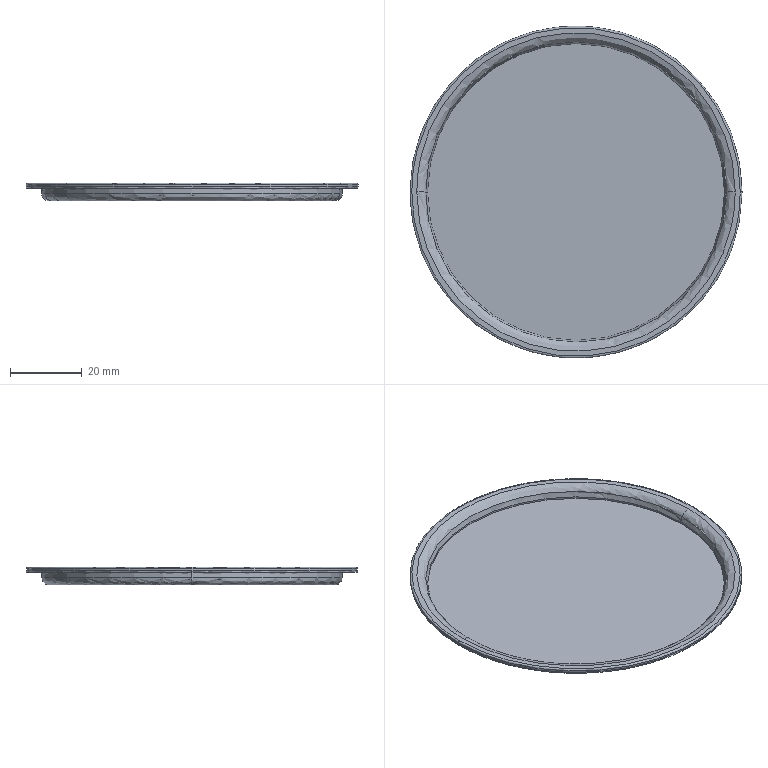Part | SolidWorks | features BaseBody 1 | 1 solid | 18 faces | box 92.8 x 92.8 x 5 mm | volume 9835 mm3 | spline 8 | cylinder 6 | plane 4 | commonest cylinder face diameters 83 x2 84 x2 92.8 x2
STEP:
#1=CARTESIAN_POINT('',(41.5,0.,2.));
#2=VERTEX_POINT('',#1);
#3=CARTESIAN_POINT('',(-41.5,0.,2.));
#4=VERTEX_POINT('',#3);
#5=CARTESIAN_POINT('',(0.,0.,2.));
#6=DIRECTION('',(0.,0.,-1.));
#7=DIRECTION('',(1.,0.,0.));
#8=AXIS2_PLACEMENT_3D('',#5,#6,#7);
#9=CIRCLE('',#8,41.5);
#10=EDGE_CURVE('',#2,#4,#9,.T.);
#11=ORIENTED_EDGE('',*,*,#10,.T.);
#12=CARTESIAN_POINT('',(-44.5,0.,5.));
#13=VERTEX_POINT('',#12);
#14=CARTESIAN_POINT('',(-44.5,0.,2.));
#15=DIRECTION('',(0.,-1.,0.));
#16=DIRECTION('',(-1.,0.,0.));
#17=AXIS2_PLACEMENT_3D('',#14,#15,#16);
#18=CIRCLE('',#17,3.);
#19=EDGE_CURVE('',#4,#13,#18,.T.);
#20=ORIENTED_EDGE('',*,*,#19,.T.);
#21=CARTESIAN_POINT('',(44.5,0.,5.));
#22=VERTEX_POINT('',#21);
#23=CARTESIAN_POINT('',(-44.5,0.,5.));
#24=CARTESIAN_POINT('',(-44.5,-89.,5.));
#25=CARTESIAN_POINT('',(44.5,-89.,5.));
#26=CARTESIAN_POINT('',(44.5,0.,5.));
#27=(BOUNDED_CURVE()B_SPLINE_CURVE(3,(#23,#24,#25,#26),.UNSPECIFIED.,.F.,.F.)B_SPLINE_CURVE_WITH_KNOTS((4,4),(0.,1.),.UNSPECIFIED.)CURVE()GEOMETRIC_REPRESENTATION_ITEM()RATIONAL_B_SPLINE_CURVE((1.,0.3333,0.3333,1.))REPRESENTATION_ITEM(''));
#28=EDGE_CURVE('',#13,#22,#27,.T.);
#29=ORIENTED_EDGE('',*,*,#28,.T.);
#30=CARTESIAN_POINT('',(44.5,0.,2.));
#31=DIRECTION('',(0.,1.,0.));
#32=DIRECTION('',(1.,0.,0.));
#33=AXIS2_PLACEMENT_3D('',#30,#31,#32);
#34=CIRCLE('',#33,3.);
#35=EDGE_CURVE('',#2,#22,#34,.T.);
#36=ORIENTED_EDGE('',*,*,#35,.F.);
#37=EDGE_LOOP('',(#11,#20,#29,#36));
#38=FACE_OUTER_BOUND('',#37,.T.);
#39=CARTESIAN_POINT('',(-41.5,0.,2.));
#40=CARTESIAN_POINT('',(-41.5,-83.,2.));
#41=CARTESIAN_POINT('',(41.5,-83.,2.));
#42=CARTESIAN_POINT('',(41.5,0.,2.));
#43=CARTESIAN_POINT('',(-41.5,0.,3.757));
#44=CARTESIAN_POINT('',(-41.5,-83.,3.757));
#45=CARTESIAN_POINT('',(41.5,-83.,3.757));
#46=CARTESIAN_POINT('',(41.5,0.,3.757));
#47=CARTESIAN_POINT('',(-42.743,0.,5.));
#48=CARTESIAN_POINT('',(-42.743,-85.485,5.));
#49=CARTESIAN_POINT('',(42.743,-85.485,5.));
#50=CARTESIAN_POINT('',(42.743,0.,5.));
#51=CARTESIAN_POINT('',(-44.5,0.,5.));
#52=CARTESIAN_POINT('',(-44.5,-89.,5.));
#53=CARTESIAN_POINT('',(44.5,-89.,5.));
#54=CARTESIAN_POINT('',(44.5,0.,5.));
#55=(BOUNDED_SURFACE()B_SPLINE_SURFACE(3,3,((#39,#40,#41,#42),(#43,#44,#45,#46),(#47,#48,#49,#50),(#51,#52,#53,#54)),.UNSPECIFIED.,.F.,.F.,.F.)B_SPLINE_SURFACE_WITH_KNOTS((4,4),(4,4),(0.,1.),(0.,1.),.UNSPECIFIED.)GEOMETRIC_REPRESENTATION_ITEM()RATIONAL_B_SPLINE_SURFACE(((1.,0.3333,0.3333,1.),(0.8047,0.2682,0.2682,0.8047),(0.8047,0.2682,0.2682,0.8047),(1.,0.3333,0.3333,1.)))REPRESENTATION_ITEM('')SURFACE());
#56=ADVANCED_FACE('',(#38),#55,.T.);
#57=CARTESIAN_POINT('',(-45.9,0.,5.));
#58=VERTEX_POINT('',#57);
#59=CARTESIAN_POINT('',(45.9,0.,5.));
#60=VERTEX_POINT('',#59);
#61=CARTESIAN_POINT('',(-45.9,0.,5.));
#62=CARTESIAN_POINT('',(-45.9,-1.404,5.));
#63=CARTESIAN_POINT('',(-45.804,-3.5,5.));
#64=CARTESIAN_POINT('',(-45.525,-5.931,5.));
#65=CARTESIAN_POINT('',(-45.343,-7.143,5.));
#66=CARTESIAN_POINT('',(-45.242,-7.748,5.));
#67=CARTESIAN_POINT('',(-45.189,-8.05,5.));
#68=CARTESIAN_POINT('',(-45.161,-8.201,5.));
#69=CARTESIAN_POINT('',(-45.15,-8.266,5.));
#70=CARTESIAN_POINT('',(-45.142,-8.309,5.));
#71=CARTESIAN_POINT('',(-45.138,-8.329,5.));
#72=CARTESIAN_POINT('',(-44.863,-9.816,5.));
#73=CARTESIAN_POINT('',(-44.353,-11.981,5.));
#74=CARTESIAN_POINT('',(-43.576,-14.456,5.));
#75=CARTESIAN_POINT('',(-43.142,-15.68,5.));
#76=CARTESIAN_POINT('',(-42.913,-16.289,5.));
#77=CARTESIAN_POINT('',(-42.796,-16.592,5.));
#78=CARTESIAN_POINT('',(-42.745,-16.722,5.));
#79=CARTESIAN_POINT('',(-42.711,-16.809,5.));
#80=CARTESIAN_POINT('',(-42.695,-16.85,5.));
#81=CARTESIAN_POINT('',(-42.106,-18.338,5.));
#82=CARTESIAN_POINT('',(-41.146,-20.447,5.));
#83=CARTESIAN_POINT('',(-39.843,-22.813,5.));
#84=CARTESIAN_POINT('',(-39.146,-23.973,5.));
#85=CARTESIAN_POINT('',(-38.786,-24.547,5.));
#86=CARTESIAN_POINT('',(-38.629,-24.792,5.));
#87=CARTESIAN_POINT('',(-38.524,-24.954,5.));
#88=CARTESIAN_POINT('',(-38.472,-25.034,5.));
#89=CARTESIAN_POINT('',(-36.684,-27.769,5.));
#90=CARTESIAN_POINT('',(-34.697,-30.216,5.));
#91=CARTESIAN_POINT('',(-31.336,-33.576,5.));
#92=CARTESIAN_POINT('',(-29.578,-35.162,5.));
#93=CARTESIAN_POINT('',(-27.393,-36.845,5.));
#94=CARTESIAN_POINT('',(-26.266,-37.646,5.));
#95=CARTESIAN_POINT('',(-25.694,-38.035,5.));
#96=CARTESIAN_POINT('',(-25.447,-38.2,5.));
#97=CARTESIAN_POINT('',(-25.283,-38.309,5.));
#98=CARTESIAN_POINT('',(-25.198,-38.365,5.));
#99=CARTESIAN_POINT('',(-23.819,-39.267,5.));
#100=CARTESIAN_POINT('',(-21.818,-40.436,5.));
#101=CARTESIAN_POINT('',(-19.388,-41.617,5.));
#102=CARTESIAN_POINT('',(-18.15,-42.162,5.));
#103=CARTESIAN_POINT('',(-17.525,-42.424,5.));
#104=CARTESIAN_POINT('',(-17.211,-42.551,5.));
#105=CARTESIAN_POINT('',(-17.076,-42.606,5.));
#106=CARTESIAN_POINT('',(-16.986,-42.642,5.));
#107=CARTESIAN_POINT('',(-16.939,-42.66,5.));
#108=CARTESIAN_POINT('',(-15.512,-43.225,5.));
#109=CARTESIAN_POINT('',(-13.406,-43.943,5.));
#110=CARTESIAN_POINT('',(-10.896,-44.599,5.));
#111=CARTESIAN_POINT('',(-9.629,-44.882,5.));
#112=CARTESIAN_POINT('',(-8.991,-45.011,5.));
#113=CARTESIAN_POINT('',(-8.672,-45.074,5.));
#114=CARTESIAN_POINT('',(-8.512,-45.104,5.));
#115=CARTESIAN_POINT('',(-8.444,-45.117,5.));
#116=CARTESIAN_POINT('',(-8.398,-45.125,5.));
#117=CARTESIAN_POINT('',(-8.374,-45.13,5.));
#118=CARTESIAN_POINT('',(-5.592,-45.645,5.));
#119=CARTESIAN_POINT('',(-2.807,-45.9,5.));
#120=CARTESIAN_POINT('',(1.404,-45.9,5.));
#121=CARTESIAN_POINT('',(3.5,-45.804,5.));
#122=CARTESIAN_POINT('',(5.931,-45.525,5.));
#123=CARTESIAN_POINT('',(7.143,-45.343,5.));
#124=CARTESIAN_POINT('',(7.748,-45.242,5.));
#125=CARTESIAN_POINT('',(8.05,-45.189,5.));
#126=CARTESIAN_POINT('',(8.201,-45.161,5.));
#127=CARTESIAN_POINT('',(8.266,-45.15,5.));
#128=CARTESIAN_POINT('',(8.309,-45.142,5.));
#129=CARTESIAN_POINT('',(8.329,-45.138,5.));
#130=CARTESIAN_POINT('',(9.816,-44.863,5.));
#131=CARTESIAN_POINT('',(11.981,-44.353,5.));
#132=CARTESIAN_POINT('',(14.456,-43.576,5.));
#133=CARTESIAN_POINT('',(15.68,-43.142,5.));
#134=CARTESIAN_POINT('',(16.289,-42.913,5.));
#135=CARTESIAN_POINT('',(16.592,-42.796,5.));
#136=CARTESIAN_POINT('',(16.722,-42.745,5.));
#137=CARTESIAN_POINT('',(16.809,-42.711,5.));
#138=CARTESIAN_POINT('',(16.85,-42.695,5.));
#139=CARTESIAN_POINT('',(18.338,-42.106,5.));
#140=CARTESIAN_POINT('',(20.447,-41.146,5.));
#141=CARTESIAN_POINT('',(22.813,-39.843,5.));
#142=CARTESIAN_POINT('',(23.973,-39.146,5.));
#143=CARTESIAN_POINT('',(24.547,-38.786,5.));
#144=CARTESIAN_POINT('',(24.792,-38.629,5.));
#145=CARTESIAN_POINT('',(24.954,-38.524,5.));
#146=CARTESIAN_POINT('',(25.034,-38.472,5.));
#147=CARTESIAN_POINT('',(27.769,-36.684,5.));
#148=CARTESIAN_POINT('',(30.216,-34.697,5.));
#149=CARTESIAN_POINT('',(33.576,-31.336,5.));
#150=CARTESIAN_POINT('',(35.162,-29.578,5.));
#151=CARTESIAN_POINT('',(36.845,-27.393,5.));
#152=CARTESIAN_POINT('',(37.646,-26.266,5.));
#153=CARTESIAN_POINT('',(38.035,-25.694,5.));
#154=CARTESIAN_POINT('',(38.2,-25.447,5.));
#155=CARTESIAN_POINT('',(38.309,-25.283,5.));
#156=CARTESIAN_POINT('',(38.365,-25.198,5.));
#157=CARTESIAN_POINT('',(39.267,-23.819,5.));
#158=CARTESIAN_POINT('',(40.436,-21.818,5.));
#159=CARTESIAN_POINT('',(41.617,-19.388,5.));
#160=CARTESIAN_POINT('',(42.162,-18.15,5.));
#161=CARTESIAN_POINT('',(42.424,-17.525,5.));
#162=CARTESIAN_POINT('',(42.551,-17.211,5.));
#163=CARTESIAN_POINT('',(42.606,-17.076,5.));
#164=CARTESIAN_POINT('',(42.642,-16.986,5.));
#165=CARTESIAN_POINT('',(42.66,-16.939,5.));
#166=CARTESIAN_POINT('',(43.225,-15.512,5.));
#167=CARTESIAN_POINT('',(43.943,-13.406,5.));
#168=CARTESIAN_POINT('',(44.599,-10.896,5.));
#169=CARTESIAN_POINT('',(44.882,-9.629,5.));
#170=CARTESIAN_POINT('',(45.011,-8.991,5.));
#171=CARTESIAN_POINT('',(45.074,-8.672,5.));
#172=CARTESIAN_POINT('',(45.104,-8.512,5.));
#173=CARTESIAN_POINT('',(45.117,-8.444,5.));
#174=CARTESIAN_POINT('',(45.125,-8.398,5.));
#175=CARTESIAN_POINT('',(45.13,-8.374,5.));
#176=CARTESIAN_POINT('',(45.645,-5.592,5.));
#177=CARTESIAN_POINT('',(45.9,-2.808,5.));
#178=CARTESIAN_POINT('',(45.9,0.,5.));
#179=B_SPLINE_CURVE_WITH_KNOTS('',3,(#61,#62,#63,#64,#65,#66,#67,#68,#69,#70,#71,#72,#73,#74,#75,#76,#77,#78,#79,#80,#81,#82,#83,#84,#85,#86,#87,#88,#89,#90,#91,#92,#93,#94,#95,#96,#97,#98,#99,#100,#101,#102,#103,#104,#105,#106,#107,#108,#109,#110,#111,#112,#113,#114,#115,#116,#117,#118,#119,#120,#121,#122,#123,#124,#125,#126,#127,#128,#129,#130,#131,#132,#133,#134,#135,#136,#137,#138,#139,#140,#141,#142,#143,#144,#145,#146,#147,#148,#149,#150,#151,#152,#153,#154,#155,#156,#157,#158,#159,#160,#161,#162,#163,#164,#165,#166,#167,#168,#169,#170,#171,#172,#173,#174,#175,#176,#177,#178),.UNSPECIFIED.,.F.,.F.,(4,1,1,1,1,1,1,2,2,1,1,1,1,1,2,2,1,1,1,1,2,2,2,1,1,1,1,2,2,1,1,1,1,1,2,2,1,1,1,1,1,1,2,2,2,1,1,1,1,1,1,2,2,1,1,1,1,1,2,2,1,1,1,1,2,2,2,1,1,1,1,2,2,1,1,1,1,1,2,2,1,1,1,1,1,1,2,2,4),(0.,0.03125,0.04687,0.05469,0.05859,0.06055,0.06152,0.06201,0.0625,0.09375,0.1094,0.1172,0.1211,0.123,0.124,0.125,0.1562,0.1719,0.1797,0.1836,0.1855,0.1875,0.25,0.2812,0.2969,0.3047,0.3086,0.3105,0.3125,0.3437,0.3594,0.3672,0.3711,0.373,0.374,0.375,0.4062,0.4219,0.4297,0.4336,0.4355,0.4365,0.437,0.4375,0.5,0.5312,0.5469,0.5547,0.5586,0.5605,0.5615,0.562,0.5625,0.5937,0.6094,0.6172,0.6211,0.623,0.624,0.625,0.6562,0.6719,0.6797,0.6836,0.6855,0.6875,0.75,0.7812,0.7969,0.8047,0.8086,0.8105,0.8125,0.8437,0.8594,0.8672,0.8711,0.873,0.874,0.875,0.9062,0.9219,0.9297,0.9336,0.9355,0.9365,0.937,0.9375,1.),.UNSPECIFIED.);
#180=EDGE_CURVE('',#58,#60,#179,.T.);
#181=ORIENTED_EDGE('',*,*,#180,.F.);
#182=CARTESIAN_POINT('',(-46.4,0.,4.5));
#183=VERTEX_POINT('',#182);
#184=CARTESIAN_POINT('',(-45.9,0.,4.5));
#185=DIRECTION('',(0.,-1.,0.));
#186=DIRECTION('',(-1.,0.,0.));
#187=AXIS2_PLACEMENT_3D('',#184,#185,#186);
#188=CIRCLE('',#187,0.5);
#189=EDGE_CURVE('',#58,#183,#188,.T.);
#190=ORIENTED_EDGE('',*,*,#189,.T.);
#191=CARTESIAN_POINT('',(46.4,0.,4.5));
#192=VERTEX_POINT('',#191);
#193=CARTESIAN_POINT('',(0.,0.,4.5));
#194=DIRECTION('',(0.,0.,1.));
#195=DIRECTION('',(1.,0.,0.));
#196=AXIS2_PLACEMENT_3D('',#193,#194,#195);
#197=CIRCLE('',#196,46.4);
#198=EDGE_CURVE('',#183,#192,#197,.T.);
#199=ORIENTED_EDGE('',*,*,#198,.T.);
#200=CARTESIAN_POINT('',(45.9,0.,4.5));
#201=DIRECTION('',(0.,1.,0.));
#202=DIRECTION('',(1.,0.,0.));
#203=AXIS2_PLACEMENT_3D('',#200,#201,#202);
#204=CIRCLE('',#203,0.5);
#205=EDGE_CURVE('',#60,#192,#204,.T.);
#206=ORIENTED_EDGE('',*,*,#205,.F.);
#207=EDGE_LOOP('',(#181,#190,#199,#206));
#208=FACE_OUTER_BOUND('',#207,.T.);
#209=CARTESIAN_POINT('',(-45.9,0.,5.));
#210=CARTESIAN_POINT('',(-45.9,-91.8,5.));
#211=CARTESIAN_POINT('',(45.9,-91.8,5.));
#212=CARTESIAN_POINT('',(45.9,0.,5.));
#213=CARTESIAN_POINT('',(-46.193,0.,5.));
#214=CARTESIAN_POINT('',(-46.193,-92.386,5.));
#215=CARTESIAN_POINT('',(46.193,-92.386,5.));
#216=CARTESIAN_POINT('',(46.193,0.,5.));
#217=CARTESIAN_POINT('',(-46.4,0.,4.793));
#218=CARTESIAN_POINT('',(-46.4,-92.8,4.793));
#219=CARTESIAN_POINT('',(46.4,-92.8,4.793));
#220=CARTESIAN_POINT('',(46.4,0.,4.793));
#221=CARTESIAN_POINT('',(-46.4,0.,4.5));
#222=CARTESIAN_POINT('',(-46.4,-92.8,4.5));
#223=CARTESIAN_POINT('',(46.4,-92.8,4.5));
#224=CARTESIAN_POINT('',(46.4,0.,4.5));
#225=(BOUNDED_SURFACE()B_SPLINE_SURFACE(3,3,((#209,#210,#211,#212),(#213,#214,#215,#216),(#217,#218,#219,#220),(#221,#222,#223,#224)),.UNSPECIFIED.,.F.,.F.,.F.)B_SPLINE_SURFACE_WITH_KNOTS((4,4),(4,4),(0.,1.),(0.,1.),.UNSPECIFIED.)GEOMETRIC_REPRESENTATION_ITEM()RATIONAL_B_SPLINE_SURFACE(((1.,0.3333,0.3333,1.),(0.8047,0.2682,0.2682,0.8047),(0.8047,0.2682,0.2682,0.8047),(1.,0.3333,0.3333,1.)))REPRESENTATION_ITEM('')SURFACE());
#226=ADVANCED_FACE('',(#208),#225,.T.);
#227=CARTESIAN_POINT('',(-45.9,0.,3.5));
#228=VERTEX_POINT('',#227);
#229=CARTESIAN_POINT('',(45.9,0.,3.5));
#230=VERTEX_POINT('',#229);
#231=CARTESIAN_POINT('',(-45.9,0.,3.5));
#232=CARTESIAN_POINT('',(-45.9,-91.8,3.5));
#233=CARTESIAN_POINT('',(45.9,-91.8,3.5));
#234=CARTESIAN_POINT('',(45.9,0.,3.5));
#235=(BOUNDED_CURVE()B_SPLINE_CURVE(3,(#231,#232,#233,#234),.UNSPECIFIED.,.F.,.F.)B_SPLINE_CURVE_WITH_KNOTS((4,4),(0.,1.),.UNSPECIFIED.)CURVE()GEOMETRIC_REPRESENTATION_ITEM()RATIONAL_B_SPLINE_CURVE((1.,0.3333,0.3333,1.))REPRESENTATION_ITEM(''));
#236=EDGE_CURVE('',#228,#230,#235,.T.);
#237=ORIENTED_EDGE('',*,*,#236,.T.);
#238=CARTESIAN_POINT('',(46.4,0.,4.));
#239=VERTEX_POINT('',#238);
#240=CARTESIAN_POINT('',(45.9,0.,4.));
#241=DIRECTION('',(0.,-1.,0.));
#242=DIRECTION('',(1.,0.,0.));
#243=AXIS2_PLACEMENT_3D('',#240,#241,#242);
#244=CIRCLE('',#243,0.5);
#245=EDGE_CURVE('',#230,#239,#244,.T.);
#246=ORIENTED_EDGE('',*,*,#245,.T.);
#247=CARTESIAN_POINT('',(-46.4,0.,4.));
#248=VERTEX_POINT('',#247);
#249=CARTESIAN_POINT('',(0.,0.,4.));
#250=DIRECTION('',(0.,0.,1.));
#251=DIRECTION('',(-1.,0.,0.));
#252=AXIS2_PLACEMENT_3D('',#249,#250,#251);
#253=CIRCLE('',#252,46.4);
#254=EDGE_CURVE('',#248,#239,#253,.T.);
#255=ORIENTED_EDGE('',*,*,#254,.F.);
#256=CARTESIAN_POINT('',(-45.9,0.,4.));
#257=DIRECTION('',(0.,1.,0.));
#258=DIRECTION('',(-1.,0.,0.));
#259=AXIS2_PLACEMENT_3D('',#256,#257,#258);
#260=CIRCLE('',#259,0.5);
#261=EDGE_CURVE('',#228,#248,#260,.T.);
#262=ORIENTED_EDGE('',*,*,#261,.F.);
#263=EDGE_LOOP('',(#237,#246,#255,#262));
#264=FACE_OUTER_BOUND('',#263,.T.);
#265=CARTESIAN_POINT('',(45.9,0.,3.5));
#266=CARTESIAN_POINT('',(45.9,-91.8,3.5));
#267=CARTESIAN_POINT('',(-45.9,-91.8,3.5));
#268=CARTESIAN_POINT('',(-45.9,0.,3.5));
#269=CARTESIAN_POINT('',(46.193,0.,3.5));
#270=CARTESIAN_POINT('',(46.193,-92.386,3.5));
#271=CARTESIAN_POINT('',(-46.193,-92.386,3.5));
#272=CARTESIAN_POINT('',(-46.193,0.,3.5));
#273=CARTESIAN_POINT('',(46.4,0.,3.707));
#274=CARTESIAN_POINT('',(46.4,-92.8,3.707));
#275=CARTESIAN_POINT('',(-46.4,-92.8,3.707));
#276=CARTESIAN_POINT('',(-46.4,0.,3.707));
#277=CARTESIAN_POINT('',(46.4,0.,4.));
#278=CARTESIAN_POINT('',(46.4,-92.8,4.));
#279=CARTESIAN_POINT('',(-46.4,-92.8,4.));
#280=CARTESIAN_POINT('',(-46.4,0.,4.));
#281=(BOUNDED_SURFACE()B_SPLINE_SURFACE(3,3,((#265,#266,#267,#268),(#269,#270,#271,#272),(#273,#274,#275,#276),(#277,#278,#279,#280)),.UNSPECIFIED.,.F.,.F.,.T.)B_SPLINE_SURFACE_WITH_KNOTS((4,4),(4,4),(0.,1.),(0.,1.),.UNSPECIFIED.)GEOMETRIC_REPRESENTATION_ITEM()RATIONAL_B_SPLINE_SURFACE(((1.,0.3333,0.3333,1.),(0.8047,0.2682,0.2682,0.8047),(0.8047,0.2682,0.2682,0.8047),(1.,0.3333,0.3333,1.)))REPRESENTATION_ITEM('')SURFACE());
#282=ADVANCED_FACE('',(#264),#281,.T.);
#283=CARTESIAN_POINT('',(-42.,0.,2.));
#284=VERTEX_POINT('',#283);
#285=CARTESIAN_POINT('',(42.,0.,2.));
#286=VERTEX_POINT('',#285);
#287=CARTESIAN_POINT('',(0.,0.,2.));
#288=DIRECTION('',(0.,0.,1.));
#289=DIRECTION('',(-1.,0.,0.));
#290=AXIS2_PLACEMENT_3D('',#287,#288,#289);
#291=CIRCLE('',#290,42.);
#292=EDGE_CURVE('',#284,#286,#291,.T.);
#293=ORIENTED_EDGE('',*,*,#292,.F.);
#294=CARTESIAN_POINT('',(-40.,0.,0.));
#295=VERTEX_POINT('',#294);
#296=CARTESIAN_POINT('',(-40.,0.,2.));
#297=DIRECTION('',(0.,-1.,0.));
#298=DIRECTION('',(-1.,0.,0.));
#299=AXIS2_PLACEMENT_3D('',#296,#297,#298);
#300=CIRCLE('',#299,2.);
#301=EDGE_CURVE('',#284,#295,#300,.T.);
#302=ORIENTED_EDGE('',*,*,#301,.T.);
#303=CARTESIAN_POINT('',(40.,0.,0.));
#304=VERTEX_POINT('',#303);
#305=CARTESIAN_POINT('',(-40.,0.,0.));
#306=CARTESIAN_POINT('',(-40.,-80.,0.));
#307=CARTESIAN_POINT('',(40.,-80.,0.));
#308=CARTESIAN_POINT('',(40.,0.,0.));
#309=(BOUNDED_CURVE()B_SPLINE_CURVE(3,(#305,#306,#307,#308),.UNSPECIFIED.,.F.,.F.)B_SPLINE_CURVE_WITH_KNOTS((4,4),(0.,1.),.UNSPECIFIED.)CURVE()GEOMETRIC_REPRESENTATION_ITEM()RATIONAL_B_SPLINE_CURVE((1.,0.3333,0.3333,1.))REPRESENTATION_ITEM(''));
#310=EDGE_CURVE('',#295,#304,#309,.T.);
#311=ORIENTED_EDGE('',*,*,#310,.T.);
#312=CARTESIAN_POINT('',(40.,0.,2.));
#313=DIRECTION('',(0.,1.,0.));
#314=DIRECTION('',(1.,0.,0.));
#315=AXIS2_PLACEMENT_3D('',#312,#313,#314);
#316=CIRCLE('',#315,2.);
#317=EDGE_CURVE('',#286,#304,#316,.T.);
#318=ORIENTED_EDGE('',*,*,#317,.F.);
#319=EDGE_LOOP('',(#293,#302,#311,#318));
#320=FACE_OUTER_BOUND('',#319,.T.);
#321=CARTESIAN_POINT('',(-42.,0.,2.));
#322=CARTESIAN_POINT('',(-42.,-84.,2.));
#323=CARTESIAN_POINT('',(42.,-84.,2.));
#324=CARTESIAN_POINT('',(42.,0.,2.));
#325=CARTESIAN_POINT('',(-42.,0.,0.8284));
#326=CARTESIAN_POINT('',(-42.,-84.,0.8284));
#327=CARTESIAN_POINT('',(42.,-84.,0.8284));
#328=CARTESIAN_POINT('',(42.,0.,0.8284));
#329=CARTESIAN_POINT('',(-41.172,0.,0.));
#330=CARTESIAN_POINT('',(-41.172,-82.343,0.));
#331=CARTESIAN_POINT('',(41.172,-82.343,0.));
#332=CARTESIAN_POINT('',(41.172,0.,0.));
#333=CARTESIAN_POINT('',(-40.,0.,0.));
#334=CARTESIAN_POINT('',(-40.,-80.,0.));
#335=CARTESIAN_POINT('',(40.,-80.,0.));
#336=CARTESIAN_POINT('',(40.,0.,0.));
#337=(BOUNDED_SURFACE()B_SPLINE_SURFACE(3,3,((#321,#322,#323,#324),(#325,#326,#327,#328),(#329,#330,#331,#332),(#333,#334,#335,#336)),.UNSPECIFIED.,.F.,.F.,.T.)B_SPLINE_SURFACE_WITH_KNOTS((4,4),(4,4),(0.,1.),(0.,1.),.UNSPECIFIED.)GEOMETRIC_REPRESENTATION_ITEM()RATIONAL_B_SPLINE_SURFACE(((1.,0.3333,0.3333,1.),(0.8047,0.2682,0.2682,0.8047),(0.8047,0.2682,0.2682,0.8047),(1.,0.3333,0.3333,1.)))REPRESENTATION_ITEM('')SURFACE());
#338=ADVANCED_FACE('',(#320),#337,.T.);
#339=CARTESIAN_POINT('',(-41.5,0.,1.5));
#340=VERTEX_POINT('',#339);
#341=CARTESIAN_POINT('',(41.5,0.,1.5));
#342=VERTEX_POINT('',#341);
#343=CARTESIAN_POINT('',(0.,0.,1.5));
#344=DIRECTION('',(0.,0.,1.));
#345=DIRECTION('',(1.,0.,0.));
#346=AXIS2_PLACEMENT_3D('',#343,#344,#345);
#347=CIRCLE('',#346,41.5);
#348=EDGE_CURVE('',#340,#342,#347,.T.);
#349=ORIENTED_EDGE('',*,*,#348,.F.);
#350=CARTESIAN_POINT('',(-41.5,0.,1.5));
#351=DIRECTION('',(0.,0.,1.));
#352=VECTOR('',#351,1000.);
#353=LINE('',#350,#352);
#354=EDGE_CURVE('',#340,#4,#353,.T.);
#355=ORIENTED_EDGE('',*,*,#354,.T.);
#356=ORIENTED_EDGE('',*,*,#10,.F.);
#357=CARTESIAN_POINT('',(41.5,0.,1.5));
#358=DIRECTION('',(0.,0.,1.));
#359=VECTOR('',#358,1000.);
#360=LINE('',#357,#359);
#361=EDGE_CURVE('',#342,#2,#360,.T.);
#362=ORIENTED_EDGE('',*,*,#361,.F.);
#363=EDGE_LOOP('',(#349,#355,#356,#362));
#364=FACE_OUTER_BOUND('',#363,.T.);
#365=CARTESIAN_POINT('',(0.,0.,1.5));
#366=DIRECTION('',(0.,0.,1.));
#367=DIRECTION('',(1.,0.,0.));
#368=AXIS2_PLACEMENT_3D('',#365,#366,#367);
#369=CYLINDRICAL_SURFACE('',#368,41.5);
#370=ADVANCED_FACE('',(#364),#369,.F.);
#371=CARTESIAN_POINT('',(0.,0.,4.5));
#372=DIRECTION('',(0.,0.,1.));
#373=DIRECTION('',(1.,0.,0.));
#374=AXIS2_PLACEMENT_3D('',#371,#372,#373);
#375=CIRCLE('',#374,46.4);
#376=EDGE_CURVE('',#192,#183,#375,.T.);
#377=ORIENTED_EDGE('',*,*,#376,.F.);
#378=CARTESIAN_POINT('',(46.4,0.,5.));
#379=DIRECTION('',(0.,0.,-1.));
#380=VECTOR('',#379,1000.);
#381=LINE('',#378,#380);
#382=EDGE_CURVE('',#192,#239,#381,.T.);
#383=ORIENTED_EDGE('',*,*,#382,.T.);
#384=CARTESIAN_POINT('',(0.,0.,4.));
#385=DIRECTION('',(0.,0.,1.));
#386=DIRECTION('',(-1.,0.,0.));
#387=AXIS2_PLACEMENT_3D('',#384,#385,#386);
#388=CIRCLE('',#387,46.4);
#389=EDGE_CURVE('',#239,#248,#388,.T.);
#390=ORIENTED_EDGE('',*,*,#389,.T.);
#391=CARTESIAN_POINT('',(-46.4,0.,5.));
#392=DIRECTION('',(0.,0.,-1.));
#393=VECTOR('',#392,1000.);
#394=LINE('',#391,#393);
#395=EDGE_CURVE('',#183,#248,#394,.T.);
#396=ORIENTED_EDGE('',*,*,#395,.F.);
#397=EDGE_LOOP('',(#377,#383,#390,#396));
#398=FACE_OUTER_BOUND('',#397,.T.);
#399=CARTESIAN_POINT('',(0.,0.,5.));
#400=DIRECTION('',(0.,0.,-1.));
#401=DIRECTION('',(-1.,0.,0.));
#402=AXIS2_PLACEMENT_3D('',#399,#400,#401);
#403=CYLINDRICAL_SURFACE('',#402,46.4);
#404=ADVANCED_FACE('',(#398),#403,.T.);
#405=CARTESIAN_POINT('',(42.,0.,3.5));
#406=VERTEX_POINT('',#405);
#407=CARTESIAN_POINT('',(-42.,0.,3.5));
#408=VERTEX_POINT('',#407);
#409=CARTESIAN_POINT('',(0.,0.,3.5));
#410=DIRECTION('',(0.,0.,1.));
#411=DIRECTION('',(-1.,0.,0.));
#412=AXIS2_PLACEMENT_3D('',#409,#410,#411);
#413=CIRCLE('',#412,42.);
#414=EDGE_CURVE('',#406,#408,#413,.T.);
#415=ORIENTED_EDGE('',*,*,#414,.F.);
#416=CARTESIAN_POINT('',(42.,0.,3.5));
#417=DIRECTION('',(0.,0.,-1.));
#418=VECTOR('',#417,1000.);
#419=LINE('',#416,#418);
#420=EDGE_CURVE('',#406,#286,#419,.T.);
#421=ORIENTED_EDGE('',*,*,#420,.T.);
#422=CARTESIAN_POINT('',(0.,0.,2.));
#423=DIRECTION('',(0.,0.,1.));
#424=DIRECTION('',(-1.,0.,0.));
#425=AXIS2_PLACEMENT_3D('',#422,#423,#424);
#426=CIRCLE('',#425,42.);
#427=EDGE_CURVE('',#286,#284,#426,.T.);
#428=ORIENTED_EDGE('',*,*,#427,.T.);
#429=CARTESIAN_POINT('',(-42.,0.,3.5));
#430=DIRECTION('',(0.,0.,-1.));
#431=VECTOR('',#430,1000.);
#432=LINE('',#429,#431);
#433=EDGE_CURVE('',#408,#284,#432,.T.);
#434=ORIENTED_EDGE('',*,*,#433,.F.);
#435=EDGE_LOOP('',(#415,#421,#428,#434));
#436=FACE_OUTER_BOUND('',#435,.T.);
#437=CARTESIAN_POINT('',(0.,0.,3.5));
#438=DIRECTION('',(0.,0.,-1.));
#439=DIRECTION('',(-1.,0.,0.));
#440=AXIS2_PLACEMENT_3D('',#437,#438,#439);
#441=CYLINDRICAL_SURFACE('',#440,42.);
#442=ADVANCED_FACE('',(#436),#441,.T.);
#443=CARTESIAN_POINT('',(0.,0.,1.5));
#444=DIRECTION('',(0.,0.,1.));
#445=DIRECTION('',(1.,0.,0.));
#446=AXIS2_PLACEMENT_3D('',#443,#444,#445);
#447=CIRCLE('',#446,41.5);
#448=EDGE_CURVE('',#342,#340,#447,.T.);
#449=ORIENTED_EDGE('',*,*,#448,.T.);
#450=ORIENTED_EDGE('',*,*,#348,.T.);
#451=EDGE_LOOP('',(#449,#450));
#452=FACE_OUTER_BOUND('',#451,.T.);
#453=CARTESIAN_POINT('',(0.,0.,1.5));
#454=DIRECTION('',(0.,0.,1.));
#455=DIRECTION('',(1.,0.,0.));
#456=AXIS2_PLACEMENT_3D('',#453,#454,#455);
#457=PLANE('',#456);
#458=ADVANCED_FACE('',(#452),#457,.T.);
#459=ORIENTED_EDGE('',*,*,#354,.F.);
#460=ORIENTED_EDGE('',*,*,#448,.F.);
#461=ORIENTED_EDGE('',*,*,#361,.T.);
#462=CARTESIAN_POINT('',(0.,0.,2.));
#463=DIRECTION('',(0.,0.,-1.));
#464=DIRECTION('',(1.,0.,0.));
#465=AXIS2_PLACEMENT_3D('',#462,#463,#464);
#466=CIRCLE('',#465,41.5);
#467=EDGE_CURVE('',#4,#2,#466,.T.);
#468=ORIENTED_EDGE('',*,*,#467,.F.);
#469=EDGE_LOOP('',(#459,#460,#461,#468));
#470=FACE_OUTER_BOUND('',#469,.T.);
#471=CARTESIAN_POINT('',(0.,0.,1.5));
#472=DIRECTION('',(0.,0.,1.));
#473=DIRECTION('',(1.,0.,0.));
#474=AXIS2_PLACEMENT_3D('',#471,#472,#473);
#475=CYLINDRICAL_SURFACE('',#474,41.5);
#476=ADVANCED_FACE('',(#470),#475,.F.);
#477=ORIENTED_EDGE('',*,*,#19,.F.);
#478=ORIENTED_EDGE('',*,*,#467,.T.);
#479=ORIENTED_EDGE('',*,*,#35,.T.);
#480=CARTESIAN_POINT('',(44.5,0.,5.));
#481=CARTESIAN_POINT('',(44.5,89.,5.));
#482=CARTESIAN_POINT('',(-44.5,89.,5.));
#483=CARTESIAN_POINT('',(-44.5,0.,5.));
#484=(BOUNDED_CURVE()B_SPLINE_CURVE(3,(#480,#481,#482,#483),.UNSPECIFIED.,.F.,.T.)B_SPLINE_CURVE_WITH_KNOTS((4,4),(0.,1.),.UNSPECIFIED.)CURVE()GEOMETRIC_REPRESENTATION_ITEM()RATIONAL_B_SPLINE_CURVE((1.,0.3333,0.3333,1.))REPRESENTATION_ITEM(''));
#485=EDGE_CURVE('',#22,#13,#484,.T.);
#486=ORIENTED_EDGE('',*,*,#485,.T.);
#487=EDGE_LOOP('',(#477,#478,#479,#486));
#488=FACE_OUTER_BOUND('',#487,.T.);
#489=CARTESIAN_POINT('',(41.5,0.,2.));
#490=CARTESIAN_POINT('',(41.5,83.,2.));
#491=CARTESIAN_POINT('',(-41.5,83.,2.));
#492=CARTESIAN_POINT('',(-41.5,0.,2.));
#493=CARTESIAN_POINT('',(41.5,0.,3.757));
#494=CARTESIAN_POINT('',(41.5,83.,3.757));
#495=CARTESIAN_POINT('',(-41.5,83.,3.757));
#496=CARTESIAN_POINT('',(-41.5,0.,3.757));
#497=CARTESIAN_POINT('',(42.743,0.,5.));
#498=CARTESIAN_POINT('',(42.743,85.485,5.));
#499=CARTESIAN_POINT('',(-42.743,85.485,5.));
#500=CARTESIAN_POINT('',(-42.743,0.,5.));
#501=CARTESIAN_POINT('',(44.5,0.,5.));
#502=CARTESIAN_POINT('',(44.5,89.,5.));
#503=CARTESIAN_POINT('',(-44.5,89.,5.));
#504=CARTESIAN_POINT('',(-44.5,0.,5.));
#505=(BOUNDED_SURFACE()B_SPLINE_SURFACE(3,3,((#489,#490,#491,#492),(#493,#494,#495,#496),(#497,#498,#499,#500),(#501,#502,#503,#504)),.UNSPECIFIED.,.F.,.F.,.F.)B_SPLINE_SURFACE_WITH_KNOTS((4,4),(4,4),(0.,1.),(0.,1.),.UNSPECIFIED.)GEOMETRIC_REPRESENTATION_ITEM()RATIONAL_B_SPLINE_SURFACE(((1.,0.3333,0.3333,1.),(0.8047,0.2682,0.2682,0.8047),(0.8047,0.2682,0.2682,0.8047),(1.,0.3333,0.3333,1.)))REPRESENTATION_ITEM('')SURFACE());
#506=ADVANCED_FACE('',(#488),#505,.T.);
#507=ORIENTED_EDGE('',*,*,#28,.F.);
#508=ORIENTED_EDGE('',*,*,#485,.F.);
#509=EDGE_LOOP('',(#507,#508));
#510=FACE_BOUND('',#509,.T.);
#511=CARTESIAN_POINT('',(45.9,0.,5.));
#512=CARTESIAN_POINT('',(45.9,1.404,5.));
#513=CARTESIAN_POINT('',(45.804,3.5,5.));
#514=CARTESIAN_POINT('',(45.525,5.931,5.));
#515=CARTESIAN_POINT('',(45.343,7.143,5.));
#516=CARTESIAN_POINT('',(45.242,7.748,5.));
#517=CARTESIAN_POINT('',(45.189,8.05,5.));
#518=CARTESIAN_POINT('',(45.161,8.201,5.));
#519=CARTESIAN_POINT('',(45.15,8.266,5.));
#520=CARTESIAN_POINT('',(45.142,8.309,5.));
#521=CARTESIAN_POINT('',(45.138,8.329,5.));
#522=CARTESIAN_POINT('',(44.863,9.816,5.));
#523=CARTESIAN_POINT('',(44.353,11.981,5.));
#524=CARTESIAN_POINT('',(43.576,14.456,5.));
#525=CARTESIAN_POINT('',(43.142,15.68,5.));
#526=CARTESIAN_POINT('',(42.913,16.289,5.));
#527=CARTESIAN_POINT('',(42.796,16.592,5.));
#528=CARTESIAN_POINT('',(42.745,16.722,5.));
#529=CARTESIAN_POINT('',(42.711,16.809,5.));
#530=CARTESIAN_POINT('',(42.695,16.85,5.));
#531=CARTESIAN_POINT('',(42.106,18.338,5.));
#532=CARTESIAN_POINT('',(41.146,20.447,5.));
#533=CARTESIAN_POINT('',(39.843,22.813,5.));
#534=CARTESIAN_POINT('',(39.146,23.973,5.));
#535=CARTESIAN_POINT('',(38.786,24.547,5.));
#536=CARTESIAN_POINT('',(38.629,24.792,5.));
#537=CARTESIAN_POINT('',(38.524,24.954,5.));
#538=CARTESIAN_POINT('',(38.472,25.034,5.));
#539=CARTESIAN_POINT('',(36.684,27.769,5.));
#540=CARTESIAN_POINT('',(34.697,30.216,5.));
#541=CARTESIAN_POINT('',(31.336,33.576,5.));
#542=CARTESIAN_POINT('',(29.578,35.162,5.));
#543=CARTESIAN_POINT('',(27.393,36.845,5.));
#544=CARTESIAN_POINT('',(26.266,37.646,5.));
#545=CARTESIAN_POINT('',(25.694,38.035,5.));
#546=CARTESIAN_POINT('',(25.447,38.2,5.));
#547=CARTESIAN_POINT('',(25.283,38.309,5.));
#548=CARTESIAN_POINT('',(25.198,38.365,5.));
#549=CARTESIAN_POINT('',(23.819,39.267,5.));
#550=CARTESIAN_POINT('',(21.818,40.436,5.));
#551=CARTESIAN_POINT('',(19.388,41.617,5.));
#552=CARTESIAN_POINT('',(18.15,42.162,5.));
#553=CARTESIAN_POINT('',(17.525,42.424,5.));
#554=CARTESIAN_POINT('',(17.211,42.551,5.));
#555=CARTESIAN_POINT('',(17.076,42.606,5.));
#556=CARTESIAN_POINT('',(16.986,42.642,5.));
#557=CARTESIAN_POINT('',(16.939,42.66,5.));
#558=CARTESIAN_POINT('',(15.512,43.225,5.));
#559=CARTESIAN_POINT('',(13.406,43.943,5.));
#560=CARTESIAN_POINT('',(10.896,44.599,5.));
#561=CARTESIAN_POINT('',(9.629,44.882,5.));
#562=CARTESIAN_POINT('',(8.991,45.011,5.));
#563=CARTESIAN_POINT('',(8.672,45.074,5.));
#564=CARTESIAN_POINT('',(8.512,45.104,5.));
#565=CARTESIAN_POINT('',(8.444,45.117,5.));
#566=CARTESIAN_POINT('',(8.398,45.125,5.));
#567=CARTESIAN_POINT('',(8.374,45.13,5.));
#568=CARTESIAN_POINT('',(5.592,45.645,5.));
#569=CARTESIAN_POINT('',(2.807,45.9,5.));
#570=CARTESIAN_POINT('',(-1.404,45.9,5.));
#571=CARTESIAN_POINT('',(-3.5,45.804,5.));
#572=CARTESIAN_POINT('',(-5.931,45.525,5.));
#573=CARTESIAN_POINT('',(-7.143,45.343,5.));
#574=CARTESIAN_POINT('',(-7.748,45.242,5.));
#575=CARTESIAN_POINT('',(-8.05,45.189,5.));
#576=CARTESIAN_POINT('',(-8.201,45.161,5.));
#577=CARTESIAN_POINT('',(-8.266,45.15,5.));
#578=CARTESIAN_POINT('',(-8.309,45.142,5.));
#579=CARTESIAN_POINT('',(-8.329,45.138,5.));
#580=CARTESIAN_POINT('',(-9.816,44.863,5.));
#581=CARTESIAN_POINT('',(-11.981,44.353,5.));
#582=CARTESIAN_POINT('',(-14.456,43.576,5.));
#583=CARTESIAN_POINT('',(-15.68,43.142,5.));
#584=CARTESIAN_POINT('',(-16.289,42.913,5.));
#585=CARTESIAN_POINT('',(-16.592,42.796,5.));
#586=CARTESIAN_POINT('',(-16.722,42.745,5.));
#587=CARTESIAN_POINT('',(-16.809,42.711,5.));
#588=CARTESIAN_POINT('',(-16.85,42.695,5.));
#589=CARTESIAN_POINT('',(-18.338,42.106,5.));
#590=CARTESIAN_POINT('',(-20.447,41.146,5.));
#591=CARTESIAN_POINT('',(-22.813,39.843,5.));
#592=CARTESIAN_POINT('',(-23.973,39.146,5.));
#593=CARTESIAN_POINT('',(-24.547,38.786,5.));
#594=CARTESIAN_POINT('',(-24.792,38.629,5.));
#595=CARTESIAN_POINT('',(-24.954,38.524,5.));
#596=CARTESIAN_POINT('',(-25.034,38.472,5.));
#597=CARTESIAN_POINT('',(-27.769,36.684,5.));
#598=CARTESIAN_POINT('',(-30.216,34.697,5.));
#599=CARTESIAN_POINT('',(-33.576,31.336,5.));
#600=CARTESIAN_POINT('',(-35.162,29.578,5.));
#601=CARTESIAN_POINT('',(-36.845,27.393,5.));
#602=CARTESIAN_POINT('',(-37.646,26.266,5.));
#603=CARTESIAN_POINT('',(-38.035,25.694,5.));
#604=CARTESIAN_POINT('',(-38.2,25.447,5.));
#605=CARTESIAN_POINT('',(-38.309,25.283,5.));
#606=CARTESIAN_POINT('',(-38.365,25.198,5.));
#607=CARTESIAN_POINT('',(-39.267,23.819,5.));
#608=CARTESIAN_POINT('',(-40.436,21.818,5.));
#609=CARTESIAN_POINT('',(-41.617,19.388,5.));
#610=CARTESIAN_POINT('',(-42.162,18.15,5.));
#611=CARTESIAN_POINT('',(-42.424,17.525,5.));
#612=CARTESIAN_POINT('',(-42.551,17.211,5.));
#613=CARTESIAN_POINT('',(-42.606,17.076,5.));
#614=CARTESIAN_POINT('',(-42.642,16.986,5.));
#615=CARTESIAN_POINT('',(-42.66,16.939,5.));
#616=CARTESIAN_POINT('',(-43.225,15.512,5.));
#617=CARTESIAN_POINT('',(-43.943,13.406,5.));
#618=CARTESIAN_POINT('',(-44.599,10.896,5.));
#619=CARTESIAN_POINT('',(-44.882,9.629,5.));
#620=CARTESIAN_POINT('',(-45.011,8.991,5.));
#621=CARTESIAN_POINT('',(-45.074,8.672,5.));
#622=CARTESIAN_POINT('',(-45.104,8.512,5.));
#623=CARTESIAN_POINT('',(-45.117,8.444,5.));
#624=CARTESIAN_POINT('',(-45.125,8.398,5.));
#625=CARTESIAN_POINT('',(-45.13,8.374,5.));
#626=CARTESIAN_POINT('',(-45.645,5.592,5.));
#627=CARTESIAN_POINT('',(-45.9,2.808,5.));
#628=CARTESIAN_POINT('',(-45.9,0.,5.));
#629=B_SPLINE_CURVE_WITH_KNOTS('',3,(#511,#512,#513,#514,#515,#516,#517,#518,#519,#520,#521,#522,#523,#524,#525,#526,#527,#528,#529,#530,#531,#532,#533,#534,#535,#536,#537,#538,#539,#540,#541,#542,#543,#544,#545,#546,#547,#548,#549,#550,#551,#552,#553,#554,#555,#556,#557,#558,#559,#560,#561,#562,#563,#564,#565,#566,#567,#568,#569,#570,#571,#572,#573,#574,#575,#576,#577,#578,#579,#580,#581,#582,#583,#584,#585,#586,#587,#588,#589,#590,#591,#592,#593,#594,#595,#596,#597,#598,#599,#600,#601,#602,#603,#604,#605,#606,#607,#608,#609,#610,#611,#612,#613,#614,#615,#616,#617,#618,#619,#620,#621,#622,#623,#624,#625,#626,#627,#628),.UNSPECIFIED.,.F.,.F.,(4,1,1,1,1,1,1,2,2,1,1,1,1,1,2,2,1,1,1,1,2,2,2,1,1,1,1,2,2,1,1,1,1,1,2,2,1,1,1,1,1,1,2,2,2,1,1,1,1,1,1,2,2,1,1,1,1,1,2,2,1,1,1,1,2,2,2,1,1,1,1,2,2,1,1,1,1,1,2,2,1,1,1,1,1,1,2,2,4),(0.,0.03125,0.04688,0.05469,0.05859,0.06055,0.06152,0.06201,0.0625,0.09375,0.1094,0.1172,0.1211,0.123,0.124,0.125,0.1563,0.1719,0.1797,0.1836,0.1855,0.1875,0.25,0.2813,0.2969,0.3047,0.3086,0.3105,0.3125,0.3438,0.3594,0.3672,0.3711,0.373,0.374,0.375,0.4063,0.4219,0.4297,0.4336,0.4355,0.4365,0.437,0.4375,0.5,0.5313,0.5469,0.5547,0.5586,0.5605,0.5615,0.562,0.5625,0.5938,0.6094,0.6172,0.6211,0.623,0.624,0.625,0.6563,0.6719,0.6797,0.6836,0.6855,0.6875,0.75,0.7813,0.7969,0.8047,0.8086,0.8105,0.8125,0.8438,0.8594,0.8672,0.8711,0.873,0.874,0.875,0.9062,0.9219,0.9297,0.9336,0.9355,0.9365,0.937,0.9375,1.),.UNSPECIFIED.);
#630=EDGE_CURVE('',#60,#58,#629,.T.);
#631=ORIENTED_EDGE('',*,*,#630,.T.);
#632=ORIENTED_EDGE('',*,*,#180,.T.);
#633=EDGE_LOOP('',(#631,#632));
#634=FACE_OUTER_BOUND('',#633,.T.);
#635=CARTESIAN_POINT('',(0.,0.,5.));
#636=DIRECTION('',(0.,0.,1.));
#637=DIRECTION('',(1.,0.,0.));
#638=AXIS2_PLACEMENT_3D('',#635,#636,#637);
#639=PLANE('',#638);
#640=ADVANCED_FACE('',(#510,#634),#639,.T.);
#641=ORIENTED_EDGE('',*,*,#189,.F.);
#642=ORIENTED_EDGE('',*,*,#630,.F.);
#643=ORIENTED_EDGE('',*,*,#205,.T.);
#644=ORIENTED_EDGE('',*,*,#376,.T.);
#645=EDGE_LOOP('',(#641,#642,#643,#644));
#646=FACE_OUTER_BOUND('',#645,.T.);
#647=CARTESIAN_POINT('',(45.9,0.,5.));
#648=CARTESIAN_POINT('',(45.9,91.8,5.));
#649=CARTESIAN_POINT('',(-45.9,91.8,5.));
#650=CARTESIAN_POINT('',(-45.9,0.,5.));
#651=CARTESIAN_POINT('',(46.193,0.,5.));
#652=CARTESIAN_POINT('',(46.193,92.386,5.));
#653=CARTESIAN_POINT('',(-46.193,92.386,5.));
#654=CARTESIAN_POINT('',(-46.193,0.,5.));
#655=CARTESIAN_POINT('',(46.4,0.,4.793));
#656=CARTESIAN_POINT('',(46.4,92.8,4.793));
#657=CARTESIAN_POINT('',(-46.4,92.8,4.793));
#658=CARTESIAN_POINT('',(-46.4,0.,4.793));
#659=CARTESIAN_POINT('',(46.4,0.,4.5));
#660=CARTESIAN_POINT('',(46.4,92.8,4.5));
#661=CARTESIAN_POINT('',(-46.4,92.8,4.5));
#662=CARTESIAN_POINT('',(-46.4,0.,4.5));
#663=(BOUNDED_SURFACE()B_SPLINE_SURFACE(3,3,((#647,#648,#649,#650),(#651,#652,#653,#654),(#655,#656,#657,#658),(#659,#660,#661,#662)),.UNSPECIFIED.,.F.,.F.,.F.)B_SPLINE_SURFACE_WITH_KNOTS((4,4),(4,4),(0.,1.),(0.,1.),.UNSPECIFIED.)GEOMETRIC_REPRESENTATION_ITEM()RATIONAL_B_SPLINE_SURFACE(((1.,0.3333,0.3333,1.),(0.8047,0.2682,0.2682,0.8047),(0.8047,0.2682,0.2682,0.8047),(1.,0.3333,0.3333,1.)))REPRESENTATION_ITEM('')SURFACE());
#664=ADVANCED_FACE('',(#646),#663,.T.);
#665=ORIENTED_EDGE('',*,*,#382,.F.);
#666=ORIENTED_EDGE('',*,*,#198,.F.);
#667=ORIENTED_EDGE('',*,*,#395,.T.);
#668=ORIENTED_EDGE('',*,*,#254,.T.);
#669=EDGE_LOOP('',(#665,#666,#667,#668));
#670=FACE_OUTER_BOUND('',#669,.T.);
#671=CARTESIAN_POINT('',(0.,0.,5.));
#672=DIRECTION('',(0.,0.,-1.));
#673=DIRECTION('',(-1.,0.,0.));
#674=AXIS2_PLACEMENT_3D('',#671,#672,#673);
#675=CYLINDRICAL_SURFACE('',#674,46.4);
#676=ADVANCED_FACE('',(#670),#675,.T.);
#677=ORIENTED_EDGE('',*,*,#245,.F.);
#678=CARTESIAN_POINT('',(45.9,0.,3.5));
#679=CARTESIAN_POINT('',(45.9,91.8,3.5));
#680=CARTESIAN_POINT('',(-45.9,91.8,3.5));
#681=CARTESIAN_POINT('',(-45.9,0.,3.5));
#682=(BOUNDED_CURVE()B_SPLINE_CURVE(3,(#678,#679,#680,#681),.UNSPECIFIED.,.F.,.F.)B_SPLINE_CURVE_WITH_KNOTS((4,4),(0.,1.),.UNSPECIFIED.)CURVE()GEOMETRIC_REPRESENTATION_ITEM()RATIONAL_B_SPLINE_CURVE((1.,0.3333,0.3333,1.))REPRESENTATION_ITEM(''));
#683=EDGE_CURVE('',#230,#228,#682,.T.);
#684=ORIENTED_EDGE('',*,*,#683,.T.);
#685=ORIENTED_EDGE('',*,*,#261,.T.);
#686=ORIENTED_EDGE('',*,*,#389,.F.);
#687=EDGE_LOOP('',(#677,#684,#685,#686));
#688=FACE_OUTER_BOUND('',#687,.T.);
#689=CARTESIAN_POINT('',(-45.9,0.,3.5));
#690=CARTESIAN_POINT('',(-45.9,91.8,3.5));
#691=CARTESIAN_POINT('',(45.9,91.8,3.5));
#692=CARTESIAN_POINT('',(45.9,0.,3.5));
#693=CARTESIAN_POINT('',(-46.193,0.,3.5));
#694=CARTESIAN_POINT('',(-46.193,92.386,3.5));
#695=CARTESIAN_POINT('',(46.193,92.386,3.5));
#696=CARTESIAN_POINT('',(46.193,0.,3.5));
#697=CARTESIAN_POINT('',(-46.4,0.,3.707));
#698=CARTESIAN_POINT('',(-46.4,92.8,3.707));
#699=CARTESIAN_POINT('',(46.4,92.8,3.707));
#700=CARTESIAN_POINT('',(46.4,0.,3.707));
#701=CARTESIAN_POINT('',(-46.4,0.,4.));
#702=CARTESIAN_POINT('',(-46.4,92.8,4.));
#703=CARTESIAN_POINT('',(46.4,92.8,4.));
#704=CARTESIAN_POINT('',(46.4,0.,4.));
#705=(BOUNDED_SURFACE()B_SPLINE_SURFACE(3,3,((#689,#690,#691,#692),(#693,#694,#695,#696),(#697,#698,#699,#700),(#701,#702,#703,#704)),.UNSPECIFIED.,.F.,.F.,.F.)B_SPLINE_SURFACE_WITH_KNOTS((4,4),(4,4),(0.,1.),(0.,1.),.UNSPECIFIED.)GEOMETRIC_REPRESENTATION_ITEM()RATIONAL_B_SPLINE_SURFACE(((1.,0.3333,0.3333,1.),(0.8047,0.2682,0.2682,0.8047),(0.8047,0.2682,0.2682,0.8047),(1.,0.3333,0.3333,1.)))REPRESENTATION_ITEM('')SURFACE());
#706=ADVANCED_FACE('',(#688),#705,.T.);
#707=CARTESIAN_POINT('',(0.,0.,3.5));
#708=DIRECTION('',(0.,0.,1.));
#709=DIRECTION('',(-1.,0.,0.));
#710=AXIS2_PLACEMENT_3D('',#707,#708,#709);
#711=CIRCLE('',#710,42.);
#712=EDGE_CURVE('',#408,#406,#711,.T.);
#713=ORIENTED_EDGE('',*,*,#712,.T.);
#714=ORIENTED_EDGE('',*,*,#414,.T.);
#715=EDGE_LOOP('',(#713,#714));
#716=FACE_BOUND('',#715,.T.);
#717=ORIENTED_EDGE('',*,*,#683,.F.);
#718=ORIENTED_EDGE('',*,*,#236,.F.);
#719=EDGE_LOOP('',(#717,#718));
#720=FACE_OUTER_BOUND('',#719,.T.);
#721=CARTESIAN_POINT('',(0.,0.,3.5));
#722=DIRECTION('',(0.,0.,-1.));
#723=DIRECTION('',(-1.,0.,0.));
#724=AXIS2_PLACEMENT_3D('',#721,#722,#723);
#725=PLANE('',#724);
#726=ADVANCED_FACE('',(#716,#720),#725,.T.);
#727=ORIENTED_EDGE('',*,*,#420,.F.);
#728=ORIENTED_EDGE('',*,*,#712,.F.);
#729=ORIENTED_EDGE('',*,*,#433,.T.);
#730=ORIENTED_EDGE('',*,*,#292,.T.);
#731=EDGE_LOOP('',(#727,#728,#729,#730));
#732=FACE_OUTER_BOUND('',#731,.T.);
#733=CARTESIAN_POINT('',(0.,0.,3.5));
#734=DIRECTION('',(0.,0.,-1.));
#735=DIRECTION('',(-1.,0.,0.));
#736=AXIS2_PLACEMENT_3D('',#733,#734,#735);
#737=CYLINDRICAL_SURFACE('',#736,42.);
#738=ADVANCED_FACE('',(#732),#737,.T.);
#739=ORIENTED_EDGE('',*,*,#301,.F.);
#740=ORIENTED_EDGE('',*,*,#427,.F.);
#741=ORIENTED_EDGE('',*,*,#317,.T.);
#742=CARTESIAN_POINT('',(40.,0.,0.));
#743=CARTESIAN_POINT('',(40.,80.,0.));
#744=CARTESIAN_POINT('',(-40.,80.,0.));
#745=CARTESIAN_POINT('',(-40.,0.,0.));
#746=(BOUNDED_CURVE()B_SPLINE_CURVE(3,(#742,#743,#744,#745),.UNSPECIFIED.,.F.,.F.)B_SPLINE_CURVE_WITH_KNOTS((4,4),(0.,1.),.UNSPECIFIED.)CURVE()GEOMETRIC_REPRESENTATION_ITEM()RATIONAL_B_SPLINE_CURVE((1.,0.3333,0.3333,1.))REPRESENTATION_ITEM(''));
#747=EDGE_CURVE('',#304,#295,#746,.T.);
#748=ORIENTED_EDGE('',*,*,#747,.T.);
#749=EDGE_LOOP('',(#739,#740,#741,#748));
#750=FACE_OUTER_BOUND('',#749,.T.);
#751=CARTESIAN_POINT('',(42.,0.,2.));
#752=CARTESIAN_POINT('',(42.,84.,2.));
#753=CARTESIAN_POINT('',(-42.,84.,2.));
#754=CARTESIAN_POINT('',(-42.,0.,2.));
#755=CARTESIAN_POINT('',(42.,0.,0.8284));
#756=CARTESIAN_POINT('',(42.,84.,0.8284));
#757=CARTESIAN_POINT('',(-42.,84.,0.8284));
#758=CARTESIAN_POINT('',(-42.,0.,0.8284));
#759=CARTESIAN_POINT('',(41.172,0.,0.));
#760=CARTESIAN_POINT('',(41.172,82.343,0.));
#761=CARTESIAN_POINT('',(-41.172,82.343,0.));
#762=CARTESIAN_POINT('',(-41.172,0.,0.));
#763=CARTESIAN_POINT('',(40.,0.,0.));
#764=CARTESIAN_POINT('',(40.,80.,0.));
#765=CARTESIAN_POINT('',(-40.,80.,0.));
#766=CARTESIAN_POINT('',(-40.,0.,0.));
#767=(BOUNDED_SURFACE()B_SPLINE_SURFACE(3,3,((#751,#752,#753,#754),(#755,#756,#757,#758),(#759,#760,#761,#762),(#763,#764,#765,#766)),.UNSPECIFIED.,.F.,.F.,.T.)B_SPLINE_SURFACE_WITH_KNOTS((4,4),(4,4),(0.,1.),(0.,1.),.UNSPECIFIED.)GEOMETRIC_REPRESENTATION_ITEM()RATIONAL_B_SPLINE_SURFACE(((1.,0.3333,0.3333,1.),(0.8047,0.2682,0.2682,0.8047),(0.8047,0.2682,0.2682,0.8047),(1.,0.3333,0.3333,1.)))REPRESENTATION_ITEM('')SURFACE());
#768=ADVANCED_FACE('',(#750),#767,.T.);
#769=ORIENTED_EDGE('',*,*,#747,.F.);
#770=ORIENTED_EDGE('',*,*,#310,.F.);
#771=EDGE_LOOP('',(#769,#770));
#772=FACE_OUTER_BOUND('',#771,.T.);
#773=CARTESIAN_POINT('',(0.,0.,0.));
#774=DIRECTION('',(0.,0.,1.));
#775=DIRECTION('',(1.,0.,0.));
#776=AXIS2_PLACEMENT_3D('',#773,#774,#775);
#777=PLANE('',#776);
#778=ADVANCED_FACE('',(#772),#777,.F.);
#779=CLOSED_SHELL('',(#56,#226,#282,#338,#370,#404,#442,#458,#476,#506,#640,#664,#676,#706,#726,#738,#768,#778));
#780=MANIFOLD_SOLID_BREP('',#779);
#781=CARTESIAN_POINT('',(0.,0.,0.));
#782=DIRECTION('',(0.,0.,1.));
#783=DIRECTION('',(1.,0.,0.));
#784=AXIS2_PLACEMENT_3D('',#781,#782,#783);
#785=(LENGTH_UNIT()NAMED_UNIT(*)SI_UNIT(.MILLI.,.METRE.));
#786=UNCERTAINTY_MEASURE_WITH_UNIT(LENGTH_MEASURE(0.00001),#785,'','');
#787=(NAMED_UNIT(*)PLANE_ANGLE_UNIT()SI_UNIT($,.RADIAN.));
#788=(NAMED_UNIT(*)SI_UNIT($,.STERADIAN.)SOLID_ANGLE_UNIT());
#789=(GEOMETRIC_REPRESENTATION_CONTEXT(3)GLOBAL_UNCERTAINTY_ASSIGNED_CONTEXT((#786))GLOBAL_UNIT_ASSIGNED_CONTEXT((#785,#787,#788))REPRESENTATION_CONTEXT('',''));
#790=ADVANCED_BREP_SHAPE_REPRESENTATION('',(#780,#784),#789);